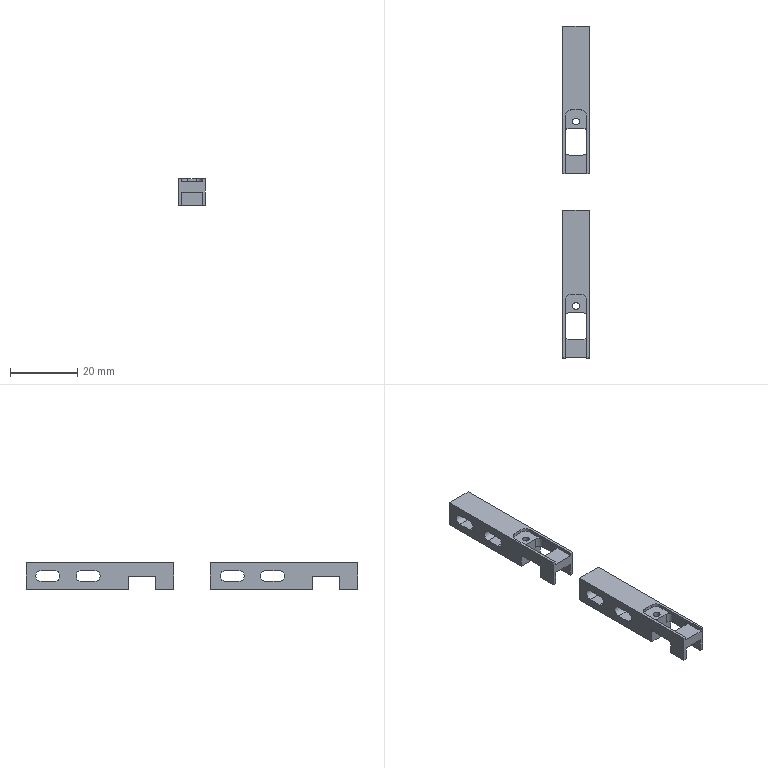CAM job | NX | 3+2 milling, drilling | part box 8 x 99 x 8 mm | stock box 10 x 104 x 10 mm
Tools:
number,name,description,diameter,corner_radius,flute_length,length,flutes
4,D4,平底铣刀-粗,4.0,0.0,25.0,75.0,2
9,D10,平底铣刀-粗,10.0,0.0,35.0,75.0,2
17,D2-J,平底铣刀-精,2.0,0.0,50.0,75.0,2
11,D3-J,平底铣刀-精,3.0,0.0,50.0,75.0,2
11,D4-J,平底铣刀-精,4.0,0.0,50.0,75.0,2
7,D6-J,平底铣刀-精,6.0,0.0,25.0,75.0,2
1,D80R0.8飞刀,圆鼻刀-粗,80.0,0.8,50.0,75.0,2
1,D80R0.8飞刀-J,圆鼻刀-精,80.0,0.8,50.0,75.0,2
2,D6倒角刀,倒角刀,6.0,0.0,3.0,25.0,2
19,M2.5X0.45,丝锥,2.05,0.0,35.0,50.0,2
17,ZT2.1,钻头,2.1,0.0,35.0,50.0,2
Operations:
program,operation,operation_type,tool,method,geometry_group,spindle_rpm,surface_speed,feed_per_tooth,feed_cut,feed_plunge,cut_length_mm,path_length_mm,cut_time_min,machine_time_min
C,盲腰槽粗,VolumeBased25DMillingOperation,D4,METHOD,W-C,9000.0,113.097,0.0667,1200.0,100.0,685.781,901.281,0.5715,0.593
C,腰槽粗_1,VolumeBased25DMillingOperation,D2-J,METHOD,W-C,12000.0,75.398,0.025,600.0,100.0,1696.565,1928.065,2.828,2.851
C,C0.3封闭铣廓倒角6X45L_COPY,PlanarMilling,D6倒角刀,爬面_倒角-切深0-步距G,W-C,7000.0,131.0,0.1071,1500.0,100.0,71.369,277.998,0.0476,0.0682
C,腰槽精,VolumeBased25DMillingOperation,D4-J,METHOD,W-C,8000.0,100.531,0.0312,500.0,100.0,33.023,254.62,0.066,0.0882
C,腰槽精_3,VolumeBased25DMillingOperation,D2-J,METHOD,W-C,6000.0,113.0,0.0167,200.0,100.0,111.986,384.786,0.5599,0.5872
B,底壁铣飞面一刀开粗_COPY,VolumeBased25DMillingOperation,D80R0.8飞刀,分层开粗-切深K-步距G,W-B,4500.0,1130.973,0.2222,2000.0,100.0,1035.97,2220.508,0.518,0.6364
B,底壁铣飞面一刀精光_COPY,VolumeBased25DMillingOperation,D80R0.8飞刀-J,侧刃精光-切深K-步距G,W-B,4500.0,1130.973,0.1111,1000.0,100.0,206.998,302.998,0.207,0.2166
B,底壁铣分层开粗-中_COPY,VolumeBased25DMillingOperation,D4,分层开粗-切深K-步距G,W-B,8000.0,100.528,0.125,2000.0,100.0,295.8,403.726,0.1479,0.1587
B,钻倒角_3,Operation,D6倒角刀,METHOD,W-B,5000.0,94.248,0.015,150.0,0.0,8.65,177.382,0.0577,0.0745
B,平面去毛刺6X45L_COPY,SurfaceContour,D6倒角刀,爬面_倒角-切深0-步距G,W-B,6500.0,122.519,0.1154,1500.0,100.0,361.456,685.693,0.241,0.2734
B,底壁铣精光侧面-中-选底面_COPY,VolumeBased25DMillingOperation,D4-J,侧刃精光-切深K-步距G,W-B,8000.0,100.528,0.05,800.0,100.0,90.383,174.988,0.113,0.1214
A,顶面_2,FaceMilling,D80R0.8飞刀,侧刃精光-切深K-步距G,W-A,4500.0,1385.0,0.1667,1500.0,100.0,193.0,289.0,0.1287,0.1383
A,外形粗_3,VolumeBased25DMillingOperation,D10,METHOD,W-A,8000.0,251.327,0.375,6000.0,80.0,3268.11,3535.61,0.5447,0.5714
A,打点-深0.8_2,Operation,D6倒角刀,NONE,W-A,8000.0,150.796,0.0312,500.0,90.0,3.6,163.209,0.0072,0.0232
A,通孔-M2.5螺纹底孔_2,Operation,ZT2.1,NONE,W-A,3000.0,19.321,0.0333,200.0,90.0,24.0,204.009,0.12,0.138
A,底壁粗_2,VolumeBased25DMillingOperation,D4,METHOD,W-A,12000.0,113.097,0.0417,1000.0,100.0,2288.0,3821.999,2.288,2.441
A,底壁铣螺旋开粗-中_COPY,VolumeBased25DMillingOperation,D4,分层开粗-切深K-步距G,W-A,8000.0,100.528,0.125,2000.0,100.0,701.165,966.284,0.3506,0.3771
A,底壁铣精光底面-中_COPY,VolumeBased25DMillingOperation,D3-J,精光步距切深关,W-A,7000.0,175.0,0.0536,1500.0,100.0,125.103,333.328,0.0834,0.1042
A,底侧精_5,VolumeBased25DMillingOperation,D3-J,METHOD,W-A,8000.0,75.398,0.05,800.0,100.0,95.85,581.61,0.1198,0.1684
A,底壁铣螺旋精光-中_COPY,VolumeBased25DMillingOperation,D3-J,螺旋精光-切深K-步距G,W-A,8000.0,75.396,0.0375,600.0,100.0,310.653,572.211,0.5178,0.5439
A,仅选体_2,SurfaceContour,D6倒角刀,METHOD,W-A,8000.0,150.796,0.1875,3000.0,100.0,309.889,995.932,0.1033,0.1719
A,钻倒角_2,Operation,D6倒角刀,METHOD,W-A,8000.0,150.796,0.0312,500.0,0.0,8.95,175.982,0.0179,0.0346
A,通孔-攻牙M2.5_2,Operation,M2.5X0.45,METHOD,W-A,1000.0,6.44,0.0002,0.45,90.0,22.0,200.009,48.889,48.907
A,外形半精_3,VolumeBased25DMillingOperation,D6-J,METHOD,W-A,9000.0,169.646,0.0667,1200.0,100.0,255.532,543.049,0.2129,0.2417